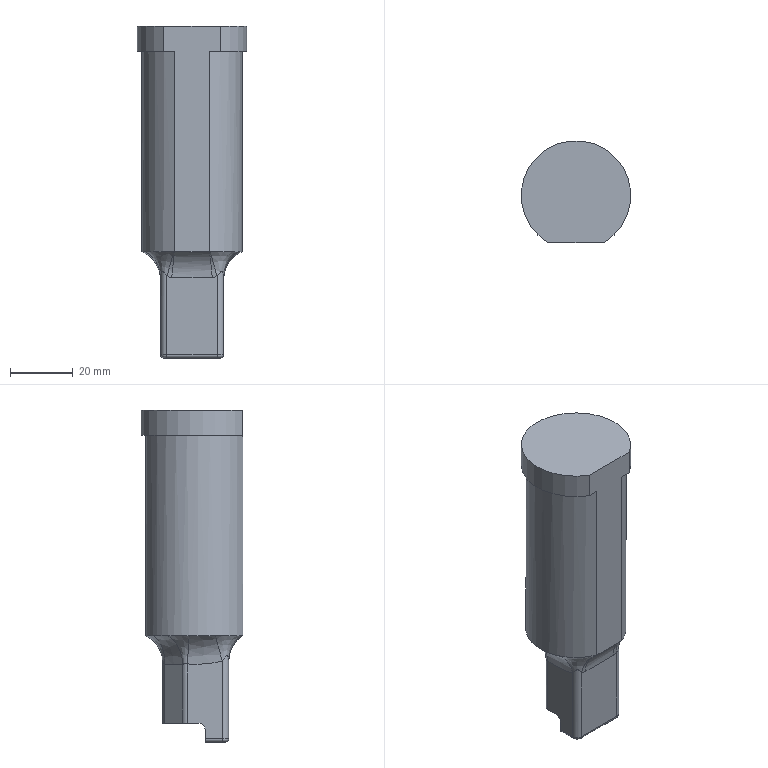Part | NX | features 8 2 | 1 solid | 36 faces | box 35 x 32.5 x 106 mm | volume 71330 mm3 | cylinder 12 | plane 11 | spline 11 | torus 2 | commonest cylinder face diameters 4 x5 2 x4 20 x1 32 x1 35 x1